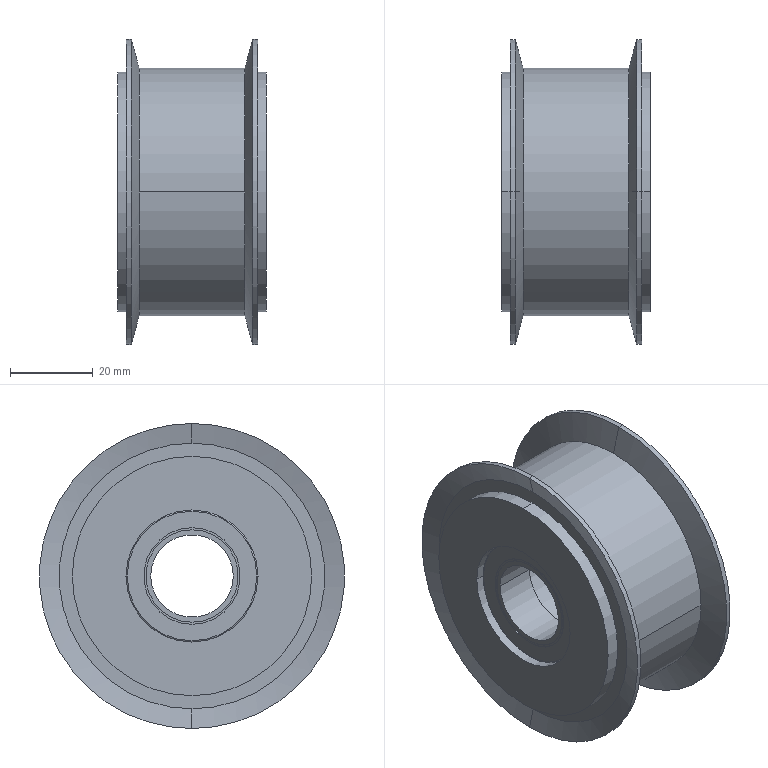Part | SolidWorks | features BaseBody 1 | 1 solid | 62 faces | box 36 x 73.9 x 73.9 mm | volume 85906 mm3 | cylinder 32 | plane 14 | torus 8 | cone 8 | commonest cylinder face diameters 32 x8 20 x4 22.4 x4 23.4 x4 58 x4 73.9 x4